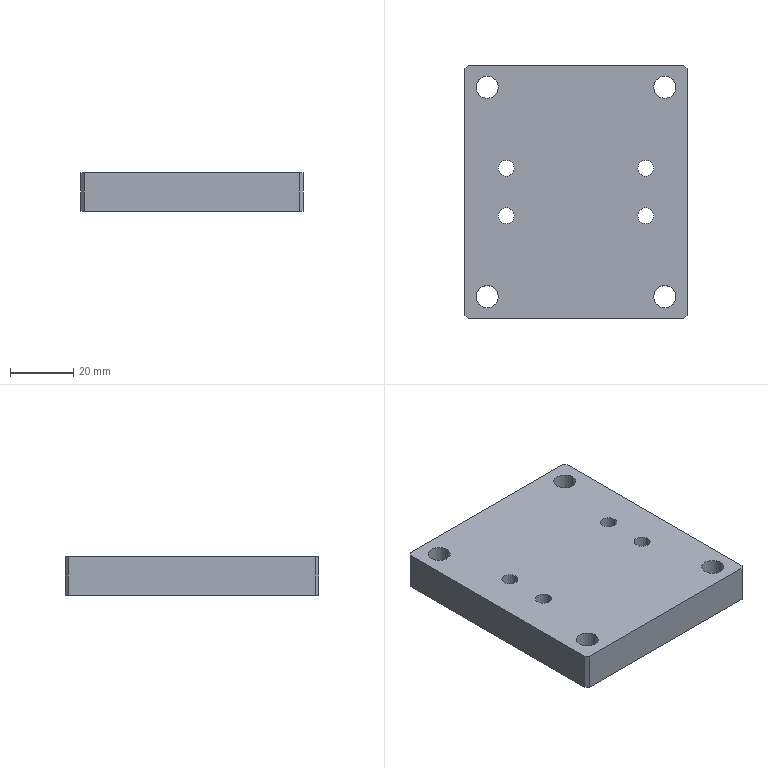Part | SolidWorks | features HoleWzd 2, Chamfer 1, Extrusion 1, ICE 1, LPattern 1 | 1 solid | 26 faces | box 70 x 80 x 12 mm | volume 64386 mm3 | cylinder 16 | plane 10 | commonest cylinder face diameters 5 x8 7 x8
STEP:
#1=CARTESIAN_POINT('',(59.5,-32.5,12.));
#2=VERTEX_POINT('',#1);
#3=CARTESIAN_POINT('',(54.5,-32.5,12.));
#4=VERTEX_POINT('',#3);
#5=CARTESIAN_POINT('',(57.,-32.5,12.));
#6=DIRECTION('',(0.,0.,-1.));
#7=DIRECTION('',(-1.,0.,0.));
#8=AXIS2_PLACEMENT_3D('',#5,#6,#7);
#9=CIRCLE('',#8,2.5);
#10=EDGE_CURVE('',#2,#4,#9,.T.);
#11=ORIENTED_EDGE('',*,*,#10,.F.);
#12=CARTESIAN_POINT('',(59.5,-32.5,0.));
#13=VERTEX_POINT('',#12);
#14=CARTESIAN_POINT('',(59.5,-32.5,0.));
#15=DIRECTION('',(0.,0.,-1.));
#16=VECTOR('',#15,1000.);
#17=LINE('',#14,#16);
#18=EDGE_CURVE('',#2,#13,#17,.T.);
#19=ORIENTED_EDGE('',*,*,#18,.T.);
#20=CARTESIAN_POINT('',(54.5,-32.5,0.));
#21=VERTEX_POINT('',#20);
#22=CARTESIAN_POINT('',(57.,-32.5,0.));
#23=DIRECTION('',(0.,0.,-1.));
#24=DIRECTION('',(-1.,0.,0.));
#25=AXIS2_PLACEMENT_3D('',#22,#23,#24);
#26=CIRCLE('',#25,2.5);
#27=EDGE_CURVE('',#13,#21,#26,.T.);
#28=ORIENTED_EDGE('',*,*,#27,.T.);
#29=CARTESIAN_POINT('',(54.5,-32.5,0.));
#30=DIRECTION('',(0.,0.,-1.));
#31=VECTOR('',#30,1000.);
#32=LINE('',#29,#31);
#33=EDGE_CURVE('',#4,#21,#32,.T.);
#34=ORIENTED_EDGE('',*,*,#33,.F.);
#35=EDGE_LOOP('',(#11,#19,#28,#34));
#36=FACE_OUTER_BOUND('',#35,.T.);
#37=CARTESIAN_POINT('',(57.,-32.5,0.));
#38=DIRECTION('',(0.,0.,-1.));
#39=DIRECTION('',(-1.,0.,0.));
#40=AXIS2_PLACEMENT_3D('',#37,#38,#39);
#41=CYLINDRICAL_SURFACE('',#40,2.5);
#42=ADVANCED_FACE('',(#36),#41,.F.);
#43=CARTESIAN_POINT('',(59.5,-47.5,12.));
#44=VERTEX_POINT('',#43);
#45=CARTESIAN_POINT('',(54.5,-47.5,12.));
#46=VERTEX_POINT('',#45);
#47=CARTESIAN_POINT('',(57.,-47.5,12.));
#48=DIRECTION('',(0.,0.,-1.));
#49=DIRECTION('',(-1.,0.,0.));
#50=AXIS2_PLACEMENT_3D('',#47,#48,#49);
#51=CIRCLE('',#50,2.5);
#52=EDGE_CURVE('',#44,#46,#51,.T.);
#53=ORIENTED_EDGE('',*,*,#52,.F.);
#54=CARTESIAN_POINT('',(59.5,-47.5,0.));
#55=VERTEX_POINT('',#54);
#56=CARTESIAN_POINT('',(59.5,-47.5,0.));
#57=DIRECTION('',(0.,0.,-1.));
#58=VECTOR('',#57,1000.);
#59=LINE('',#56,#58);
#60=EDGE_CURVE('',#44,#55,#59,.T.);
#61=ORIENTED_EDGE('',*,*,#60,.T.);
#62=CARTESIAN_POINT('',(54.5,-47.5,0.));
#63=VERTEX_POINT('',#62);
#64=CARTESIAN_POINT('',(57.,-47.5,0.));
#65=DIRECTION('',(0.,0.,-1.));
#66=DIRECTION('',(-1.,0.,0.));
#67=AXIS2_PLACEMENT_3D('',#64,#65,#66);
#68=CIRCLE('',#67,2.5);
#69=EDGE_CURVE('',#55,#63,#68,.T.);
#70=ORIENTED_EDGE('',*,*,#69,.T.);
#71=CARTESIAN_POINT('',(54.5,-47.5,0.));
#72=DIRECTION('',(0.,0.,-1.));
#73=VECTOR('',#72,1000.);
#74=LINE('',#71,#73);
#75=EDGE_CURVE('',#46,#63,#74,.T.);
#76=ORIENTED_EDGE('',*,*,#75,.F.);
#77=EDGE_LOOP('',(#53,#61,#70,#76));
#78=FACE_OUTER_BOUND('',#77,.T.);
#79=CARTESIAN_POINT('',(57.,-47.5,0.));
#80=DIRECTION('',(0.,0.,-1.));
#81=DIRECTION('',(-1.,0.,0.));
#82=AXIS2_PLACEMENT_3D('',#79,#80,#81);
#83=CYLINDRICAL_SURFACE('',#82,2.5);
#84=ADVANCED_FACE('',(#78),#83,.F.);
#85=CARTESIAN_POINT('',(15.5,-47.5,12.));
#86=VERTEX_POINT('',#85);
#87=CARTESIAN_POINT('',(10.5,-47.5,12.));
#88=VERTEX_POINT('',#87);
#89=CARTESIAN_POINT('',(13.,-47.5,12.));
#90=DIRECTION('',(0.,0.,-1.));
#91=DIRECTION('',(-1.,0.,0.));
#92=AXIS2_PLACEMENT_3D('',#89,#90,#91);
#93=CIRCLE('',#92,2.5);
#94=EDGE_CURVE('',#86,#88,#93,.T.);
#95=ORIENTED_EDGE('',*,*,#94,.F.);
#96=CARTESIAN_POINT('',(15.5,-47.5,0.));
#97=VERTEX_POINT('',#96);
#98=CARTESIAN_POINT('',(15.5,-47.5,0.));
#99=DIRECTION('',(0.,0.,-1.));
#100=VECTOR('',#99,1000.);
#101=LINE('',#98,#100);
#102=EDGE_CURVE('',#86,#97,#101,.T.);
#103=ORIENTED_EDGE('',*,*,#102,.T.);
#104=CARTESIAN_POINT('',(10.5,-47.5,0.));
#105=VERTEX_POINT('',#104);
#106=CARTESIAN_POINT('',(13.,-47.5,0.));
#107=DIRECTION('',(0.,0.,-1.));
#108=DIRECTION('',(-1.,0.,0.));
#109=AXIS2_PLACEMENT_3D('',#106,#107,#108);
#110=CIRCLE('',#109,2.5);
#111=EDGE_CURVE('',#97,#105,#110,.T.);
#112=ORIENTED_EDGE('',*,*,#111,.T.);
#113=CARTESIAN_POINT('',(10.5,-47.5,0.));
#114=DIRECTION('',(0.,0.,-1.));
#115=VECTOR('',#114,1000.);
#116=LINE('',#113,#115);
#117=EDGE_CURVE('',#88,#105,#116,.T.);
#118=ORIENTED_EDGE('',*,*,#117,.F.);
#119=EDGE_LOOP('',(#95,#103,#112,#118));
#120=FACE_OUTER_BOUND('',#119,.T.);
#121=CARTESIAN_POINT('',(13.,-47.5,0.));
#122=DIRECTION('',(0.,0.,-1.));
#123=DIRECTION('',(-1.,0.,0.));
#124=AXIS2_PLACEMENT_3D('',#121,#122,#123);
#125=CYLINDRICAL_SURFACE('',#124,2.5);
#126=ADVANCED_FACE('',(#120),#125,.F.);
#127=CARTESIAN_POINT('',(15.5,-32.5,12.));
#128=VERTEX_POINT('',#127);
#129=CARTESIAN_POINT('',(10.5,-32.5,12.));
#130=VERTEX_POINT('',#129);
#131=CARTESIAN_POINT('',(13.,-32.5,12.));
#132=DIRECTION('',(0.,0.,-1.));
#133=DIRECTION('',(-1.,0.,0.));
#134=AXIS2_PLACEMENT_3D('',#131,#132,#133);
#135=CIRCLE('',#134,2.5);
#136=EDGE_CURVE('',#128,#130,#135,.T.);
#137=ORIENTED_EDGE('',*,*,#136,.F.);
#138=CARTESIAN_POINT('',(15.5,-32.5,0.));
#139=VERTEX_POINT('',#138);
#140=CARTESIAN_POINT('',(15.5,-32.5,0.));
#141=DIRECTION('',(0.,0.,-1.));
#142=VECTOR('',#141,1000.);
#143=LINE('',#140,#142);
#144=EDGE_CURVE('',#128,#139,#143,.T.);
#145=ORIENTED_EDGE('',*,*,#144,.T.);
#146=CARTESIAN_POINT('',(10.5,-32.5,0.));
#147=VERTEX_POINT('',#146);
#148=CARTESIAN_POINT('',(13.,-32.5,0.));
#149=DIRECTION('',(0.,0.,-1.));
#150=DIRECTION('',(-1.,0.,0.));
#151=AXIS2_PLACEMENT_3D('',#148,#149,#150);
#152=CIRCLE('',#151,2.5);
#153=EDGE_CURVE('',#139,#147,#152,.T.);
#154=ORIENTED_EDGE('',*,*,#153,.T.);
#155=CARTESIAN_POINT('',(10.5,-32.5,0.));
#156=DIRECTION('',(0.,0.,-1.));
#157=VECTOR('',#156,1000.);
#158=LINE('',#155,#157);
#159=EDGE_CURVE('',#130,#147,#158,.T.);
#160=ORIENTED_EDGE('',*,*,#159,.F.);
#161=EDGE_LOOP('',(#137,#145,#154,#160));
#162=FACE_OUTER_BOUND('',#161,.T.);
#163=CARTESIAN_POINT('',(13.,-32.5,0.));
#164=DIRECTION('',(0.,0.,-1.));
#165=DIRECTION('',(-1.,0.,0.));
#166=AXIS2_PLACEMENT_3D('',#163,#164,#165);
#167=CYLINDRICAL_SURFACE('',#166,2.5);
#168=ADVANCED_FACE('',(#162),#167,.F.);
#169=CARTESIAN_POINT('',(10.5,-73.,12.));
#170=VERTEX_POINT('',#169);
#171=CARTESIAN_POINT('',(3.5,-73.,12.));
#172=VERTEX_POINT('',#171);
#173=CARTESIAN_POINT('',(7.,-73.,12.));
#174=DIRECTION('',(0.,0.,-1.));
#175=DIRECTION('',(-1.,0.,0.));
#176=AXIS2_PLACEMENT_3D('',#173,#174,#175);
#177=CIRCLE('',#176,3.5);
#178=EDGE_CURVE('',#170,#172,#177,.T.);
#179=ORIENTED_EDGE('',*,*,#178,.F.);
#180=CARTESIAN_POINT('',(10.5,-73.,0.));
#181=VERTEX_POINT('',#180);
#182=CARTESIAN_POINT('',(10.5,-73.,0.));
#183=DIRECTION('',(0.,0.,-1.));
#184=VECTOR('',#183,1000.);
#185=LINE('',#182,#184);
#186=EDGE_CURVE('',#170,#181,#185,.T.);
#187=ORIENTED_EDGE('',*,*,#186,.T.);
#188=CARTESIAN_POINT('',(3.5,-73.,0.));
#189=VERTEX_POINT('',#188);
#190=CARTESIAN_POINT('',(7.,-73.,0.));
#191=DIRECTION('',(0.,0.,-1.));
#192=DIRECTION('',(-1.,0.,0.));
#193=AXIS2_PLACEMENT_3D('',#190,#191,#192);
#194=CIRCLE('',#193,3.5);
#195=EDGE_CURVE('',#181,#189,#194,.T.);
#196=ORIENTED_EDGE('',*,*,#195,.T.);
#197=CARTESIAN_POINT('',(3.5,-73.,0.));
#198=DIRECTION('',(0.,0.,-1.));
#199=VECTOR('',#198,1000.);
#200=LINE('',#197,#199);
#201=EDGE_CURVE('',#172,#189,#200,.T.);
#202=ORIENTED_EDGE('',*,*,#201,.F.);
#203=EDGE_LOOP('',(#179,#187,#196,#202));
#204=FACE_OUTER_BOUND('',#203,.T.);
#205=CARTESIAN_POINT('',(7.,-73.,0.));
#206=DIRECTION('',(0.,0.,-1.));
#207=DIRECTION('',(-1.,0.,0.));
#208=AXIS2_PLACEMENT_3D('',#205,#206,#207);
#209=CYLINDRICAL_SURFACE('',#208,3.5);
#210=ADVANCED_FACE('',(#204),#209,.F.);
#211=CARTESIAN_POINT('',(10.5,-7.,12.));
#212=VERTEX_POINT('',#211);
#213=CARTESIAN_POINT('',(3.5,-7.,12.));
#214=VERTEX_POINT('',#213);
#215=CARTESIAN_POINT('',(7.,-7.,12.));
#216=DIRECTION('',(0.,0.,-1.));
#217=DIRECTION('',(-1.,0.,0.));
#218=AXIS2_PLACEMENT_3D('',#215,#216,#217);
#219=CIRCLE('',#218,3.5);
#220=EDGE_CURVE('',#212,#214,#219,.T.);
#221=ORIENTED_EDGE('',*,*,#220,.F.);
#222=CARTESIAN_POINT('',(10.5,-7.,0.));
#223=VERTEX_POINT('',#222);
#224=CARTESIAN_POINT('',(10.5,-7.,0.));
#225=DIRECTION('',(0.,0.,-1.));
#226=VECTOR('',#225,1000.);
#227=LINE('',#224,#226);
#228=EDGE_CURVE('',#212,#223,#227,.T.);
#229=ORIENTED_EDGE('',*,*,#228,.T.);
#230=CARTESIAN_POINT('',(3.5,-7.,0.));
#231=VERTEX_POINT('',#230);
#232=CARTESIAN_POINT('',(7.,-7.,0.));
#233=DIRECTION('',(0.,0.,-1.));
#234=DIRECTION('',(-1.,0.,0.));
#235=AXIS2_PLACEMENT_3D('',#232,#233,#234);
#236=CIRCLE('',#235,3.5);
#237=EDGE_CURVE('',#223,#231,#236,.T.);
#238=ORIENTED_EDGE('',*,*,#237,.T.);
#239=CARTESIAN_POINT('',(3.5,-7.,0.));
#240=DIRECTION('',(0.,0.,-1.));
#241=VECTOR('',#240,1000.);
#242=LINE('',#239,#241);
#243=EDGE_CURVE('',#214,#231,#242,.T.);
#244=ORIENTED_EDGE('',*,*,#243,.F.);
#245=EDGE_LOOP('',(#221,#229,#238,#244));
#246=FACE_OUTER_BOUND('',#245,.T.);
#247=CARTESIAN_POINT('',(7.,-7.,0.));
#248=DIRECTION('',(0.,0.,-1.));
#249=DIRECTION('',(-1.,0.,0.));
#250=AXIS2_PLACEMENT_3D('',#247,#248,#249);
#251=CYLINDRICAL_SURFACE('',#250,3.5);
#252=ADVANCED_FACE('',(#246),#251,.F.);
#253=CARTESIAN_POINT('',(66.5,-73.,12.));
#254=VERTEX_POINT('',#253);
#255=CARTESIAN_POINT('',(59.5,-73.,12.));
#256=VERTEX_POINT('',#255);
#257=CARTESIAN_POINT('',(63.,-73.,12.));
#258=DIRECTION('',(0.,0.,-1.));
#259=DIRECTION('',(-1.,0.,0.));
#260=AXIS2_PLACEMENT_3D('',#257,#258,#259);
#261=CIRCLE('',#260,3.5);
#262=EDGE_CURVE('',#254,#256,#261,.T.);
#263=ORIENTED_EDGE('',*,*,#262,.F.);
#264=CARTESIAN_POINT('',(66.5,-73.,0.));
#265=VERTEX_POINT('',#264);
#266=CARTESIAN_POINT('',(66.5,-73.,0.));
#267=DIRECTION('',(0.,0.,-1.));
#268=VECTOR('',#267,1000.);
#269=LINE('',#266,#268);
#270=EDGE_CURVE('',#254,#265,#269,.T.);
#271=ORIENTED_EDGE('',*,*,#270,.T.);
#272=CARTESIAN_POINT('',(59.5,-73.,0.));
#273=VERTEX_POINT('',#272);
#274=CARTESIAN_POINT('',(63.,-73.,0.));
#275=DIRECTION('',(0.,0.,-1.));
#276=DIRECTION('',(-1.,0.,0.));
#277=AXIS2_PLACEMENT_3D('',#274,#275,#276);
#278=CIRCLE('',#277,3.5);
#279=EDGE_CURVE('',#265,#273,#278,.T.);
#280=ORIENTED_EDGE('',*,*,#279,.T.);
#281=CARTESIAN_POINT('',(59.5,-73.,0.));
#282=DIRECTION('',(0.,0.,-1.));
#283=VECTOR('',#282,1000.);
#284=LINE('',#281,#283);
#285=EDGE_CURVE('',#256,#273,#284,.T.);
#286=ORIENTED_EDGE('',*,*,#285,.F.);
#287=EDGE_LOOP('',(#263,#271,#280,#286));
#288=FACE_OUTER_BOUND('',#287,.T.);
#289=CARTESIAN_POINT('',(63.,-73.,0.));
#290=DIRECTION('',(0.,0.,-1.));
#291=DIRECTION('',(-1.,0.,0.));
#292=AXIS2_PLACEMENT_3D('',#289,#290,#291);
#293=CYLINDRICAL_SURFACE('',#292,3.5);
#294=ADVANCED_FACE('',(#288),#293,.F.);
#295=CARTESIAN_POINT('',(66.5,-7.,12.));
#296=VERTEX_POINT('',#295);
#297=CARTESIAN_POINT('',(59.5,-7.,12.));
#298=VERTEX_POINT('',#297);
#299=CARTESIAN_POINT('',(63.,-7.,12.));
#300=DIRECTION('',(0.,0.,-1.));
#301=DIRECTION('',(-1.,0.,0.));
#302=AXIS2_PLACEMENT_3D('',#299,#300,#301);
#303=CIRCLE('',#302,3.5);
#304=EDGE_CURVE('',#296,#298,#303,.T.);
#305=ORIENTED_EDGE('',*,*,#304,.F.);
#306=CARTESIAN_POINT('',(66.5,-7.,0.));
#307=VERTEX_POINT('',#306);
#308=CARTESIAN_POINT('',(66.5,-7.,0.));
#309=DIRECTION('',(0.,0.,-1.));
#310=VECTOR('',#309,1000.);
#311=LINE('',#308,#310);
#312=EDGE_CURVE('',#296,#307,#311,.T.);
#313=ORIENTED_EDGE('',*,*,#312,.T.);
#314=CARTESIAN_POINT('',(59.5,-7.,0.));
#315=VERTEX_POINT('',#314);
#316=CARTESIAN_POINT('',(63.,-7.,0.));
#317=DIRECTION('',(0.,0.,-1.));
#318=DIRECTION('',(-1.,0.,0.));
#319=AXIS2_PLACEMENT_3D('',#316,#317,#318);
#320=CIRCLE('',#319,3.5);
#321=EDGE_CURVE('',#307,#315,#320,.T.);
#322=ORIENTED_EDGE('',*,*,#321,.T.);
#323=CARTESIAN_POINT('',(59.5,-7.,0.));
#324=DIRECTION('',(0.,0.,-1.));
#325=VECTOR('',#324,1000.);
#326=LINE('',#323,#325);
#327=EDGE_CURVE('',#298,#315,#326,.T.);
#328=ORIENTED_EDGE('',*,*,#327,.F.);
#329=EDGE_LOOP('',(#305,#313,#322,#328));
#330=FACE_OUTER_BOUND('',#329,.T.);
#331=CARTESIAN_POINT('',(63.,-7.,0.));
#332=DIRECTION('',(0.,0.,-1.));
#333=DIRECTION('',(-1.,0.,0.));
#334=AXIS2_PLACEMENT_3D('',#331,#332,#333);
#335=CYLINDRICAL_SURFACE('',#334,3.5);
#336=ADVANCED_FACE('',(#330),#335,.F.);
#337=CARTESIAN_POINT('',(0.,-1.,0.));
#338=VERTEX_POINT('',#337);
#339=CARTESIAN_POINT('',(0.,-79.,0.));
#340=VERTEX_POINT('',#339);
#341=CARTESIAN_POINT('',(0.,0.,0.));
#342=DIRECTION('',(0.,-1.,0.));
#343=VECTOR('',#342,1000.);
#344=LINE('',#341,#343);
#345=EDGE_CURVE('',#338,#340,#344,.T.);
#346=ORIENTED_EDGE('',*,*,#345,.T.);
#347=CARTESIAN_POINT('',(0.,-79.,12.));
#348=VERTEX_POINT('',#347);
#349=CARTESIAN_POINT('',(0.,-79.,12.));
#350=DIRECTION('',(0.,0.,1.));
#351=VECTOR('',#350,1000.);
#352=LINE('',#349,#351);
#353=EDGE_CURVE('',#340,#348,#352,.T.);
#354=ORIENTED_EDGE('',*,*,#353,.T.);
#355=CARTESIAN_POINT('',(0.,-1.,12.));
#356=VERTEX_POINT('',#355);
#357=CARTESIAN_POINT('',(0.,0.,12.));
#358=DIRECTION('',(0.,-1.,0.));
#359=VECTOR('',#358,1000.);
#360=LINE('',#357,#359);
#361=EDGE_CURVE('',#356,#348,#360,.T.);
#362=ORIENTED_EDGE('',*,*,#361,.F.);
#363=CARTESIAN_POINT('',(0.,-1.,12.));
#364=DIRECTION('',(0.,0.,-1.));
#365=VECTOR('',#364,1000.);
#366=LINE('',#363,#365);
#367=EDGE_CURVE('',#356,#338,#366,.T.);
#368=ORIENTED_EDGE('',*,*,#367,.T.);
#369=EDGE_LOOP('',(#346,#354,#362,#368));
#370=FACE_OUTER_BOUND('',#369,.T.);
#371=CARTESIAN_POINT('',(0.,0.,12.));
#372=DIRECTION('',(1.,0.,0.));
#373=DIRECTION('',(0.,1.,0.));
#374=AXIS2_PLACEMENT_3D('',#371,#372,#373);
#375=PLANE('',#374);
#376=ADVANCED_FACE('',(#370),#375,.F.);
#377=CARTESIAN_POINT('',(1.,-80.,12.));
#378=VERTEX_POINT('',#377);
#379=CARTESIAN_POINT('',(69.,-80.,12.));
#380=VERTEX_POINT('',#379);
#381=CARTESIAN_POINT('',(0.,-80.,12.));
#382=DIRECTION('',(1.,0.,0.));
#383=VECTOR('',#382,1000.);
#384=LINE('',#381,#383);
#385=EDGE_CURVE('',#378,#380,#384,.T.);
#386=ORIENTED_EDGE('',*,*,#385,.F.);
#387=CARTESIAN_POINT('',(1.,-80.,0.));
#388=VERTEX_POINT('',#387);
#389=CARTESIAN_POINT('',(1.,-80.,12.));
#390=DIRECTION('',(0.,0.,-1.));
#391=VECTOR('',#390,1000.);
#392=LINE('',#389,#391);
#393=EDGE_CURVE('',#378,#388,#392,.T.);
#394=ORIENTED_EDGE('',*,*,#393,.T.);
#395=CARTESIAN_POINT('',(69.,-80.,0.));
#396=VERTEX_POINT('',#395);
#397=CARTESIAN_POINT('',(0.,-80.,0.));
#398=DIRECTION('',(1.,0.,0.));
#399=VECTOR('',#398,1000.);
#400=LINE('',#397,#399);
#401=EDGE_CURVE('',#388,#396,#400,.T.);
#402=ORIENTED_EDGE('',*,*,#401,.T.);
#403=CARTESIAN_POINT('',(69.,-80.,12.));
#404=DIRECTION('',(0.,0.,1.));
#405=VECTOR('',#404,1000.);
#406=LINE('',#403,#405);
#407=EDGE_CURVE('',#396,#380,#406,.T.);
#408=ORIENTED_EDGE('',*,*,#407,.T.);
#409=EDGE_LOOP('',(#386,#394,#402,#408));
#410=FACE_OUTER_BOUND('',#409,.T.);
#411=CARTESIAN_POINT('',(0.,-80.,12.));
#412=DIRECTION('',(0.,1.,0.));
#413=DIRECTION('',(0.,0.,1.));
#414=AXIS2_PLACEMENT_3D('',#411,#412,#413);
#415=PLANE('',#414);
#416=ADVANCED_FACE('',(#410),#415,.F.);
#417=CARTESIAN_POINT('',(70.,-79.,12.));
#418=VERTEX_POINT('',#417);
#419=CARTESIAN_POINT('',(70.,-1.,12.));
#420=VERTEX_POINT('',#419);
#421=CARTESIAN_POINT('',(70.,0.,12.));
#422=DIRECTION('',(0.,1.,0.));
#423=VECTOR('',#422,1000.);
#424=LINE('',#421,#423);
#425=EDGE_CURVE('',#418,#420,#424,.T.);
#426=ORIENTED_EDGE('',*,*,#425,.F.);
#427=CARTESIAN_POINT('',(70.,-79.,0.));
#428=VERTEX_POINT('',#427);
#429=CARTESIAN_POINT('',(70.,-79.,12.));
#430=DIRECTION('',(0.,0.,-1.));
#431=VECTOR('',#430,1000.);
#432=LINE('',#429,#431);
#433=EDGE_CURVE('',#418,#428,#432,.T.);
#434=ORIENTED_EDGE('',*,*,#433,.T.);
#435=CARTESIAN_POINT('',(70.,-1.,0.));
#436=VERTEX_POINT('',#435);
#437=CARTESIAN_POINT('',(70.,0.,0.));
#438=DIRECTION('',(0.,1.,0.));
#439=VECTOR('',#438,1000.);
#440=LINE('',#437,#439);
#441=EDGE_CURVE('',#428,#436,#440,.T.);
#442=ORIENTED_EDGE('',*,*,#441,.T.);
#443=CARTESIAN_POINT('',(70.,-1.,12.));
#444=DIRECTION('',(0.,0.,1.));
#445=VECTOR('',#444,1000.);
#446=LINE('',#443,#445);
#447=EDGE_CURVE('',#436,#420,#446,.T.);
#448=ORIENTED_EDGE('',*,*,#447,.T.);
#449=EDGE_LOOP('',(#426,#434,#442,#448));
#450=FACE_OUTER_BOUND('',#449,.T.);
#451=CARTESIAN_POINT('',(70.,0.,12.));
#452=DIRECTION('',(-1.,0.,0.));
#453=DIRECTION('',(0.,-1.,0.));
#454=AXIS2_PLACEMENT_3D('',#451,#452,#453);
#455=PLANE('',#454);
#456=ADVANCED_FACE('',(#450),#455,.F.);
#457=CARTESIAN_POINT('',(69.,0.,12.));
#458=VERTEX_POINT('',#457);
#459=CARTESIAN_POINT('',(1.,0.,12.));
#460=VERTEX_POINT('',#459);
#461=CARTESIAN_POINT('',(0.,0.,12.));
#462=DIRECTION('',(-1.,0.,0.));
#463=VECTOR('',#462,1000.);
#464=LINE('',#461,#463);
#465=EDGE_CURVE('',#458,#460,#464,.T.);
#466=ORIENTED_EDGE('',*,*,#465,.F.);
#467=CARTESIAN_POINT('',(69.,0.,0.));
#468=VERTEX_POINT('',#467);
#469=CARTESIAN_POINT('',(69.,0.,12.));
#470=DIRECTION('',(0.,0.,-1.));
#471=VECTOR('',#470,1000.);
#472=LINE('',#469,#471);
#473=EDGE_CURVE('',#458,#468,#472,.T.);
#474=ORIENTED_EDGE('',*,*,#473,.T.);
#475=CARTESIAN_POINT('',(1.,0.,0.));
#476=VERTEX_POINT('',#475);
#477=CARTESIAN_POINT('',(0.,0.,0.));
#478=DIRECTION('',(-1.,0.,0.));
#479=VECTOR('',#478,1000.);
#480=LINE('',#477,#479);
#481=EDGE_CURVE('',#468,#476,#480,.T.);
#482=ORIENTED_EDGE('',*,*,#481,.T.);
#483=CARTESIAN_POINT('',(1.,0.,12.));
#484=DIRECTION('',(0.,0.,1.));
#485=VECTOR('',#484,1000.);
#486=LINE('',#483,#485);
#487=EDGE_CURVE('',#476,#460,#486,.T.);
#488=ORIENTED_EDGE('',*,*,#487,.T.);
#489=EDGE_LOOP('',(#466,#474,#482,#488));
#490=FACE_OUTER_BOUND('',#489,.T.);
#491=CARTESIAN_POINT('',(0.,0.,12.));
#492=DIRECTION('',(0.,-1.,0.));
#493=DIRECTION('',(0.,0.,-1.));
#494=AXIS2_PLACEMENT_3D('',#491,#492,#493);
#495=PLANE('',#494);
#496=ADVANCED_FACE('',(#490),#495,.F.);
#497=CARTESIAN_POINT('',(57.,-32.5,12.));
#498=DIRECTION('',(0.,0.,-1.));
#499=DIRECTION('',(-1.,0.,0.));
#500=AXIS2_PLACEMENT_3D('',#497,#498,#499);
#501=CIRCLE('',#500,2.5);
#502=EDGE_CURVE('',#4,#2,#501,.T.);
#503=ORIENTED_EDGE('',*,*,#502,.T.);
#504=ORIENTED_EDGE('',*,*,#10,.T.);
#505=EDGE_LOOP('',(#503,#504));
#506=FACE_BOUND('',#505,.T.);
#507=CARTESIAN_POINT('',(57.,-47.5,12.));
#508=DIRECTION('',(0.,0.,-1.));
#509=DIRECTION('',(-1.,0.,0.));
#510=AXIS2_PLACEMENT_3D('',#507,#508,#509);
#511=CIRCLE('',#510,2.5);
#512=EDGE_CURVE('',#46,#44,#511,.T.);
#513=ORIENTED_EDGE('',*,*,#512,.T.);
#514=ORIENTED_EDGE('',*,*,#52,.T.);
#515=EDGE_LOOP('',(#513,#514));
#516=FACE_BOUND('',#515,.T.);
#517=CARTESIAN_POINT('',(13.,-47.5,12.));
#518=DIRECTION('',(0.,0.,-1.));
#519=DIRECTION('',(-1.,0.,0.));
#520=AXIS2_PLACEMENT_3D('',#517,#518,#519);
#521=CIRCLE('',#520,2.5);
#522=EDGE_CURVE('',#88,#86,#521,.T.);
#523=ORIENTED_EDGE('',*,*,#522,.T.);
#524=ORIENTED_EDGE('',*,*,#94,.T.);
#525=EDGE_LOOP('',(#523,#524));
#526=FACE_BOUND('',#525,.T.);
#527=CARTESIAN_POINT('',(13.,-32.5,12.));
#528=DIRECTION('',(0.,0.,-1.));
#529=DIRECTION('',(-1.,0.,0.));
#530=AXIS2_PLACEMENT_3D('',#527,#528,#529);
#531=CIRCLE('',#530,2.5);
#532=EDGE_CURVE('',#130,#128,#531,.T.);
#533=ORIENTED_EDGE('',*,*,#532,.T.);
#534=ORIENTED_EDGE('',*,*,#136,.T.);
#535=EDGE_LOOP('',(#533,#534));
#536=FACE_BOUND('',#535,.T.);
#537=CARTESIAN_POINT('',(7.,-73.,12.));
#538=DIRECTION('',(0.,0.,-1.));
#539=DIRECTION('',(-1.,0.,0.));
#540=AXIS2_PLACEMENT_3D('',#537,#538,#539);
#541=CIRCLE('',#540,3.5);
#542=EDGE_CURVE('',#172,#170,#541,.T.);
#543=ORIENTED_EDGE('',*,*,#542,.T.);
#544=ORIENTED_EDGE('',*,*,#178,.T.);
#545=EDGE_LOOP('',(#543,#544));
#546=FACE_BOUND('',#545,.T.);
#547=CARTESIAN_POINT('',(7.,-7.,12.));
#548=DIRECTION('',(0.,0.,-1.));
#549=DIRECTION('',(-1.,0.,0.));
#550=AXIS2_PLACEMENT_3D('',#547,#548,#549);
#551=CIRCLE('',#550,3.5);
#552=EDGE_CURVE('',#214,#212,#551,.T.);
#553=ORIENTED_EDGE('',*,*,#552,.T.);
#554=ORIENTED_EDGE('',*,*,#220,.T.);
#555=EDGE_LOOP('',(#553,#554));
#556=FACE_BOUND('',#555,.T.);
#557=CARTESIAN_POINT('',(63.,-73.,12.));
#558=DIRECTION('',(0.,0.,-1.));
#559=DIRECTION('',(-1.,0.,0.));
#560=AXIS2_PLACEMENT_3D('',#557,#558,#559);
#561=CIRCLE('',#560,3.5);
#562=EDGE_CURVE('',#256,#254,#561,.T.);
#563=ORIENTED_EDGE('',*,*,#562,.T.);
#564=ORIENTED_EDGE('',*,*,#262,.T.);
#565=EDGE_LOOP('',(#563,#564));
#566=FACE_BOUND('',#565,.T.);
#567=CARTESIAN_POINT('',(63.,-7.,12.));
#568=DIRECTION('',(0.,0.,-1.));
#569=DIRECTION('',(-1.,0.,0.));
#570=AXIS2_PLACEMENT_3D('',#567,#568,#569);
#571=CIRCLE('',#570,3.5);
#572=EDGE_CURVE('',#298,#296,#571,.T.);
#573=ORIENTED_EDGE('',*,*,#572,.T.);
#574=ORIENTED_EDGE('',*,*,#304,.T.);
#575=EDGE_LOOP('',(#573,#574));
#576=FACE_BOUND('',#575,.T.);
#577=ORIENTED_EDGE('',*,*,#361,.T.);
#578=CARTESIAN_POINT('',(-39.5,-39.5,12.));
#579=DIRECTION('',(0.7071,-0.7071,0.));
#580=VECTOR('',#579,1000.);
#581=LINE('',#578,#580);
#582=EDGE_CURVE('',#348,#378,#581,.T.);
#583=ORIENTED_EDGE('',*,*,#582,.T.);
#584=ORIENTED_EDGE('',*,*,#385,.T.);
#585=CARTESIAN_POINT('',(74.5,-74.5,12.));
#586=DIRECTION('',(0.7071,0.7071,0.));
#587=VECTOR('',#586,1000.);
#588=LINE('',#585,#587);
#589=EDGE_CURVE('',#380,#418,#588,.T.);
#590=ORIENTED_EDGE('',*,*,#589,.T.);
#591=ORIENTED_EDGE('',*,*,#425,.T.);
#592=CARTESIAN_POINT('',(34.5,34.5,12.));
#593=DIRECTION('',(-0.7071,0.7071,0.));
#594=VECTOR('',#593,1000.);
#595=LINE('',#592,#594);
#596=EDGE_CURVE('',#420,#458,#595,.T.);
#597=ORIENTED_EDGE('',*,*,#596,.T.);
#598=ORIENTED_EDGE('',*,*,#465,.T.);
#599=CARTESIAN_POINT('',(0.5,-0.5,12.));
#600=DIRECTION('',(-0.7071,-0.7071,0.));
#601=VECTOR('',#600,1000.);
#602=LINE('',#599,#601);
#603=EDGE_CURVE('',#460,#356,#602,.T.);
#604=ORIENTED_EDGE('',*,*,#603,.T.);
#605=EDGE_LOOP('',(#577,#583,#584,#590,#591,#597,#598,#604));
#606=FACE_OUTER_BOUND('',#605,.T.);
#607=CARTESIAN_POINT('',(0.,0.,12.));
#608=DIRECTION('',(0.,0.,1.));
#609=DIRECTION('',(1.,0.,0.));
#610=AXIS2_PLACEMENT_3D('',#607,#608,#609);
#611=PLANE('',#610);
#612=ADVANCED_FACE('',(#506,#516,#526,#536,#546,#556,#566,#576,#606),#611,.T.);
#613=CARTESIAN_POINT('',(57.,-32.5,0.));
#614=DIRECTION('',(0.,0.,-1.));
#615=DIRECTION('',(-1.,0.,0.));
#616=AXIS2_PLACEMENT_3D('',#613,#614,#615);
#617=CIRCLE('',#616,2.5);
#618=EDGE_CURVE('',#21,#13,#617,.T.);
#619=ORIENTED_EDGE('',*,*,#618,.F.);
#620=ORIENTED_EDGE('',*,*,#27,.F.);
#621=EDGE_LOOP('',(#619,#620));
#622=FACE_BOUND('',#621,.T.);
#623=CARTESIAN_POINT('',(57.,-47.5,0.));
#624=DIRECTION('',(0.,0.,-1.));
#625=DIRECTION('',(-1.,0.,0.));
#626=AXIS2_PLACEMENT_3D('',#623,#624,#625);
#627=CIRCLE('',#626,2.5);
#628=EDGE_CURVE('',#63,#55,#627,.T.);
#629=ORIENTED_EDGE('',*,*,#628,.F.);
#630=ORIENTED_EDGE('',*,*,#69,.F.);
#631=EDGE_LOOP('',(#629,#630));
#632=FACE_BOUND('',#631,.T.);
#633=CARTESIAN_POINT('',(13.,-47.5,0.));
#634=DIRECTION('',(0.,0.,-1.));
#635=DIRECTION('',(-1.,0.,0.));
#636=AXIS2_PLACEMENT_3D('',#633,#634,#635);
#637=CIRCLE('',#636,2.5);
#638=EDGE_CURVE('',#105,#97,#637,.T.);
#639=ORIENTED_EDGE('',*,*,#638,.F.);
#640=ORIENTED_EDGE('',*,*,#111,.F.);
#641=EDGE_LOOP('',(#639,#640));
#642=FACE_BOUND('',#641,.T.);
#643=CARTESIAN_POINT('',(13.,-32.5,0.));
#644=DIRECTION('',(0.,0.,-1.));
#645=DIRECTION('',(-1.,0.,0.));
#646=AXIS2_PLACEMENT_3D('',#643,#644,#645);
#647=CIRCLE('',#646,2.5);
#648=EDGE_CURVE('',#147,#139,#647,.T.);
#649=ORIENTED_EDGE('',*,*,#648,.F.);
#650=ORIENTED_EDGE('',*,*,#153,.F.);
#651=EDGE_LOOP('',(#649,#650));
#652=FACE_BOUND('',#651,.T.);
#653=CARTESIAN_POINT('',(7.,-73.,0.));
#654=DIRECTION('',(0.,0.,-1.));
#655=DIRECTION('',(-1.,0.,0.));
#656=AXIS2_PLACEMENT_3D('',#653,#654,#655);
#657=CIRCLE('',#656,3.5);
#658=EDGE_CURVE('',#189,#181,#657,.T.);
#659=ORIENTED_EDGE('',*,*,#658,.F.);
#660=ORIENTED_EDGE('',*,*,#195,.F.);
#661=EDGE_LOOP('',(#659,#660));
#662=FACE_BOUND('',#661,.T.);
#663=CARTESIAN_POINT('',(7.,-7.,0.));
#664=DIRECTION('',(0.,0.,-1.));
#665=DIRECTION('',(-1.,0.,0.));
#666=AXIS2_PLACEMENT_3D('',#663,#664,#665);
#667=CIRCLE('',#666,3.5);
#668=EDGE_CURVE('',#231,#223,#667,.T.);
#669=ORIENTED_EDGE('',*,*,#668,.F.);
#670=ORIENTED_EDGE('',*,*,#237,.F.);
#671=EDGE_LOOP('',(#669,#670));
#672=FACE_BOUND('',#671,.T.);
#673=CARTESIAN_POINT('',(63.,-73.,0.));
#674=DIRECTION('',(0.,0.,-1.));
#675=DIRECTION('',(-1.,0.,0.));
#676=AXIS2_PLACEMENT_3D('',#673,#674,#675);
#677=CIRCLE('',#676,3.5);
#678=EDGE_CURVE('',#273,#265,#677,.T.);
#679=ORIENTED_EDGE('',*,*,#678,.F.);
#680=ORIENTED_EDGE('',*,*,#279,.F.);
#681=EDGE_LOOP('',(#679,#680));
#682=FACE_BOUND('',#681,.T.);
#683=CARTESIAN_POINT('',(63.,-7.,0.));
#684=DIRECTION('',(0.,0.,-1.));
#685=DIRECTION('',(-1.,0.,0.));
#686=AXIS2_PLACEMENT_3D('',#683,#684,#685);
#687=CIRCLE('',#686,3.5);
#688=EDGE_CURVE('',#315,#307,#687,.T.);
#689=ORIENTED_EDGE('',*,*,#688,.F.);
#690=ORIENTED_EDGE('',*,*,#321,.F.);
#691=EDGE_LOOP('',(#689,#690));
#692=FACE_BOUND('',#691,.T.);
#693=ORIENTED_EDGE('',*,*,#401,.F.);
#694=CARTESIAN_POINT('',(1.,-80.,0.));
#695=DIRECTION('',(-0.7071,0.7071,0.));
#696=VECTOR('',#695,1000.);
#697=LINE('',#694,#696);
#698=EDGE_CURVE('',#388,#340,#697,.T.);
#699=ORIENTED_EDGE('',*,*,#698,.T.);
#700=ORIENTED_EDGE('',*,*,#345,.F.);
#701=CARTESIAN_POINT('',(0.,-1.,0.));
#702=DIRECTION('',(0.7071,0.7071,0.));
#703=VECTOR('',#702,1000.);
#704=LINE('',#701,#703);
#705=EDGE_CURVE('',#338,#476,#704,.T.);
#706=ORIENTED_EDGE('',*,*,#705,.T.);
#707=ORIENTED_EDGE('',*,*,#481,.F.);
#708=CARTESIAN_POINT('',(69.,0.,0.));
#709=DIRECTION('',(0.7071,-0.7071,0.));
#710=VECTOR('',#709,1000.);
#711=LINE('',#708,#710);
#712=EDGE_CURVE('',#468,#436,#711,.T.);
#713=ORIENTED_EDGE('',*,*,#712,.T.);
#714=ORIENTED_EDGE('',*,*,#441,.F.);
#715=CARTESIAN_POINT('',(70.,-79.,0.));
#716=DIRECTION('',(-0.7071,-0.7071,0.));
#717=VECTOR('',#716,1000.);
#718=LINE('',#715,#717);
#719=EDGE_CURVE('',#428,#396,#718,.T.);
#720=ORIENTED_EDGE('',*,*,#719,.T.);
#721=EDGE_LOOP('',(#693,#699,#700,#706,#707,#713,#714,#720));
#722=FACE_OUTER_BOUND('',#721,.T.);
#723=CARTESIAN_POINT('',(0.,0.,0.));
#724=DIRECTION('',(0.,0.,1.));
#725=DIRECTION('',(1.,0.,0.));
#726=AXIS2_PLACEMENT_3D('',#723,#724,#725);
#727=PLANE('',#726);
#728=ADVANCED_FACE('',(#622,#632,#642,#652,#662,#672,#682,#692,#722),#727,.F.);
#729=ORIENTED_EDGE('',*,*,#582,.F.);
#730=ORIENTED_EDGE('',*,*,#353,.F.);
#731=ORIENTED_EDGE('',*,*,#698,.F.);
#732=ORIENTED_EDGE('',*,*,#393,.F.);
#733=EDGE_LOOP('',(#729,#730,#731,#732));
#734=FACE_OUTER_BOUND('',#733,.T.);
#735=CARTESIAN_POINT('',(1.,-80.,12.));
#736=DIRECTION('',(0.7071,0.7071,0.));
#737=DIRECTION('',(0.,0.,-1.));
#738=AXIS2_PLACEMENT_3D('',#735,#736,#737);
#739=PLANE('',#738);
#740=ADVANCED_FACE('',(#734),#739,.F.);
#741=ORIENTED_EDGE('',*,*,#589,.F.);
#742=ORIENTED_EDGE('',*,*,#407,.F.);
#743=ORIENTED_EDGE('',*,*,#719,.F.);
#744=ORIENTED_EDGE('',*,*,#433,.F.);
#745=EDGE_LOOP('',(#741,#742,#743,#744));
#746=FACE_OUTER_BOUND('',#745,.T.);
#747=CARTESIAN_POINT('',(70.,-79.,12.));
#748=DIRECTION('',(-0.7071,0.7071,0.));
#749=DIRECTION('',(0.,0.,-1.));
#750=AXIS2_PLACEMENT_3D('',#747,#748,#749);
#751=PLANE('',#750);
#752=ADVANCED_FACE('',(#746),#751,.F.);
#753=ORIENTED_EDGE('',*,*,#596,.F.);
#754=ORIENTED_EDGE('',*,*,#447,.F.);
#755=ORIENTED_EDGE('',*,*,#712,.F.);
#756=ORIENTED_EDGE('',*,*,#473,.F.);
#757=EDGE_LOOP('',(#753,#754,#755,#756));
#758=FACE_OUTER_BOUND('',#757,.T.);
#759=CARTESIAN_POINT('',(69.,0.,12.));
#760=DIRECTION('',(-0.7071,-0.7071,0.));
#761=DIRECTION('',(0.,0.,-1.));
#762=AXIS2_PLACEMENT_3D('',#759,#760,#761);
#763=PLANE('',#762);
#764=ADVANCED_FACE('',(#758),#763,.F.);
#765=ORIENTED_EDGE('',*,*,#603,.F.);
#766=ORIENTED_EDGE('',*,*,#487,.F.);
#767=ORIENTED_EDGE('',*,*,#705,.F.);
#768=ORIENTED_EDGE('',*,*,#367,.F.);
#769=EDGE_LOOP('',(#765,#766,#767,#768));
#770=FACE_OUTER_BOUND('',#769,.T.);
#771=CARTESIAN_POINT('',(0.,-1.,12.));
#772=DIRECTION('',(0.7071,-0.7071,0.));
#773=DIRECTION('',(0.,0.,-1.));
#774=AXIS2_PLACEMENT_3D('',#771,#772,#773);
#775=PLANE('',#774);
#776=ADVANCED_FACE('',(#770),#775,.F.);
#777=ORIENTED_EDGE('',*,*,#312,.F.);
#778=ORIENTED_EDGE('',*,*,#572,.F.);
#779=ORIENTED_EDGE('',*,*,#327,.T.);
#780=ORIENTED_EDGE('',*,*,#688,.T.);
#781=EDGE_LOOP('',(#777,#778,#779,#780));
#782=FACE_OUTER_BOUND('',#781,.T.);
#783=CARTESIAN_POINT('',(63.,-7.,0.));
#784=DIRECTION('',(0.,0.,-1.));
#785=DIRECTION('',(-1.,0.,0.));
#786=AXIS2_PLACEMENT_3D('',#783,#784,#785);
#787=CYLINDRICAL_SURFACE('',#786,3.5);
#788=ADVANCED_FACE('',(#782),#787,.F.);
#789=ORIENTED_EDGE('',*,*,#270,.F.);
#790=ORIENTED_EDGE('',*,*,#562,.F.);
#791=ORIENTED_EDGE('',*,*,#285,.T.);
#792=ORIENTED_EDGE('',*,*,#678,.T.);
#793=EDGE_LOOP('',(#789,#790,#791,#792));
#794=FACE_OUTER_BOUND('',#793,.T.);
#795=CARTESIAN_POINT('',(63.,-73.,0.));
#796=DIRECTION('',(0.,0.,-1.));
#797=DIRECTION('',(-1.,0.,0.));
#798=AXIS2_PLACEMENT_3D('',#795,#796,#797);
#799=CYLINDRICAL_SURFACE('',#798,3.5);
#800=ADVANCED_FACE('',(#794),#799,.F.);
#801=ORIENTED_EDGE('',*,*,#228,.F.);
#802=ORIENTED_EDGE('',*,*,#552,.F.);
#803=ORIENTED_EDGE('',*,*,#243,.T.);
#804=ORIENTED_EDGE('',*,*,#668,.T.);
#805=EDGE_LOOP('',(#801,#802,#803,#804));
#806=FACE_OUTER_BOUND('',#805,.T.);
#807=CARTESIAN_POINT('',(7.,-7.,0.));
#808=DIRECTION('',(0.,0.,-1.));
#809=DIRECTION('',(-1.,0.,0.));
#810=AXIS2_PLACEMENT_3D('',#807,#808,#809);
#811=CYLINDRICAL_SURFACE('',#810,3.5);
#812=ADVANCED_FACE('',(#806),#811,.F.);
#813=ORIENTED_EDGE('',*,*,#186,.F.);
#814=ORIENTED_EDGE('',*,*,#542,.F.);
#815=ORIENTED_EDGE('',*,*,#201,.T.);
#816=ORIENTED_EDGE('',*,*,#658,.T.);
#817=EDGE_LOOP('',(#813,#814,#815,#816));
#818=FACE_OUTER_BOUND('',#817,.T.);
#819=CARTESIAN_POINT('',(7.,-73.,0.));
#820=DIRECTION('',(0.,0.,-1.));
#821=DIRECTION('',(-1.,0.,0.));
#822=AXIS2_PLACEMENT_3D('',#819,#820,#821);
#823=CYLINDRICAL_SURFACE('',#822,3.5);
#824=ADVANCED_FACE('',(#818),#823,.F.);
#825=ORIENTED_EDGE('',*,*,#144,.F.);
#826=ORIENTED_EDGE('',*,*,#532,.F.);
#827=ORIENTED_EDGE('',*,*,#159,.T.);
#828=ORIENTED_EDGE('',*,*,#648,.T.);
#829=EDGE_LOOP('',(#825,#826,#827,#828));
#830=FACE_OUTER_BOUND('',#829,.T.);
#831=CARTESIAN_POINT('',(13.,-32.5,0.));
#832=DIRECTION('',(0.,0.,-1.));
#833=DIRECTION('',(-1.,0.,0.));
#834=AXIS2_PLACEMENT_3D('',#831,#832,#833);
#835=CYLINDRICAL_SURFACE('',#834,2.5);
#836=ADVANCED_FACE('',(#830),#835,.F.);
#837=ORIENTED_EDGE('',*,*,#102,.F.);
#838=ORIENTED_EDGE('',*,*,#522,.F.);
#839=ORIENTED_EDGE('',*,*,#117,.T.);
#840=ORIENTED_EDGE('',*,*,#638,.T.);
#841=EDGE_LOOP('',(#837,#838,#839,#840));
#842=FACE_OUTER_BOUND('',#841,.T.);
#843=CARTESIAN_POINT('',(13.,-47.5,0.));
#844=DIRECTION('',(0.,0.,-1.));
#845=DIRECTION('',(-1.,0.,0.));
#846=AXIS2_PLACEMENT_3D('',#843,#844,#845);
#847=CYLINDRICAL_SURFACE('',#846,2.5);
#848=ADVANCED_FACE('',(#842),#847,.F.);
#849=ORIENTED_EDGE('',*,*,#60,.F.);
#850=ORIENTED_EDGE('',*,*,#512,.F.);
#851=ORIENTED_EDGE('',*,*,#75,.T.);
#852=ORIENTED_EDGE('',*,*,#628,.T.);
#853=EDGE_LOOP('',(#849,#850,#851,#852));
#854=FACE_OUTER_BOUND('',#853,.T.);
#855=CARTESIAN_POINT('',(57.,-47.5,0.));
#856=DIRECTION('',(0.,0.,-1.));
#857=DIRECTION('',(-1.,0.,0.));
#858=AXIS2_PLACEMENT_3D('',#855,#856,#857);
#859=CYLINDRICAL_SURFACE('',#858,2.5);
#860=ADVANCED_FACE('',(#854),#859,.F.);
#861=ORIENTED_EDGE('',*,*,#18,.F.);
#862=ORIENTED_EDGE('',*,*,#502,.F.);
#863=ORIENTED_EDGE('',*,*,#33,.T.);
#864=ORIENTED_EDGE('',*,*,#618,.T.);
#865=EDGE_LOOP('',(#861,#862,#863,#864));
#866=FACE_OUTER_BOUND('',#865,.T.);
#867=CARTESIAN_POINT('',(57.,-32.5,0.));
#868=DIRECTION('',(0.,0.,-1.));
#869=DIRECTION('',(-1.,0.,0.));
#870=AXIS2_PLACEMENT_3D('',#867,#868,#869);
#871=CYLINDRICAL_SURFACE('',#870,2.5);
#872=ADVANCED_FACE('',(#866),#871,.F.);
#873=CLOSED_SHELL('',(#42,#84,#126,#168,#210,#252,#294,#336,#376,#416,#456,#496,#612,#728,#740,#752,#764,#776,#788,#800,#812,#824,#836,#848,#860,#872));
#874=MANIFOLD_SOLID_BREP('',#873);
#875=CARTESIAN_POINT('',(0.,0.,0.));
#876=DIRECTION('',(0.,0.,1.));
#877=DIRECTION('',(1.,0.,0.));
#878=AXIS2_PLACEMENT_3D('',#875,#876,#877);
#879=(LENGTH_UNIT()NAMED_UNIT(*)SI_UNIT(.MILLI.,.METRE.));
#880=UNCERTAINTY_MEASURE_WITH_UNIT(LENGTH_MEASURE(0.00001),#879,'','');
#881=(NAMED_UNIT(*)PLANE_ANGLE_UNIT()SI_UNIT($,.RADIAN.));
#882=(NAMED_UNIT(*)SI_UNIT($,.STERADIAN.)SOLID_ANGLE_UNIT());
#883=(GEOMETRIC_REPRESENTATION_CONTEXT(3)GLOBAL_UNCERTAINTY_ASSIGNED_CONTEXT((#880))GLOBAL_UNIT_ASSIGNED_CONTEXT((#879,#881,#882))REPRESENTATION_CONTEXT('',''));
#884=ADVANCED_BREP_SHAPE_REPRESENTATION('',(#874,#878),#883);